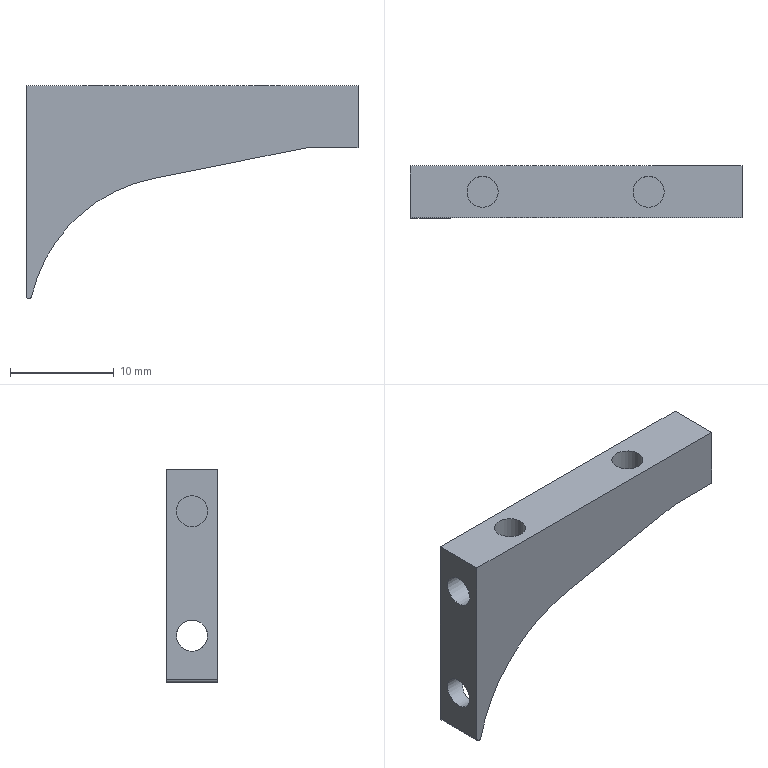Part | STEP file | 1-28.5 | 1 solid | 18 faces | box 32 x 5 x 20.5 mm | volume 1373 mm3 | plane 11 | cylinder 7 | commonest cylinder face diameters 3 x4 0.5 x2 30 x1
STEP:
#1=CARTESIAN_POINT('',(0.,0.,0.));
#2=DIRECTION('',(0.,0.,1.));
#3=DIRECTION('',(1.,0.,0.));
#4=AXIS2_PLACEMENT_3D('',#1,#2,#3);
#5=CARTESIAN_POINT('',(12.205,-2.5,11.528));
#6=VERTEX_POINT('',#5);
#7=CARTESIAN_POINT('',(27.,-2.5,14.5));
#8=VERTEX_POINT('',#7);
#9=CARTESIAN_POINT('',(12.205,-2.5,11.528));
#10=DIRECTION('',(0.9804,0.,0.1969));
#11=VECTOR('',#10,1.);
#12=LINE('',#9,#11);
#13=CARTESIAN_POINT('',(19.603,0.,13.014));
#14=DIRECTION('',(-0.1969,0.,0.9804));
#15=DIRECTION('',(0.9804,0.,0.1969));
#16=AXIS2_PLACEMENT_3D('',#13,#14,#15);
#17=PLANE('',#16);
#18=CARTESIAN_POINT('',(-7.545,-2.5));
#19=DIRECTION('',(1.,0.));
#20=VECTOR('',#19,1.);
#21=LINE('',#18,#20);
#22=(GEOMETRIC_REPRESENTATION_CONTEXT(2)PARAMETRIC_REPRESENTATION_CONTEXT()REPRESENTATION_CONTEXT('',''));
#23=DEFINITIONAL_REPRESENTATION('',(#21),#22);
#24=PCURVE('',#17,#23);
#25=CARTESIAN_POINT('',(16.,-2.5,16.));
#26=DIRECTION('',(0.,-1.,0.));
#27=DIRECTION('',(1.,0.,0.));
#28=AXIS2_PLACEMENT_3D('',#25,#26,#27);
#29=PLANE('',#28);
#30=CARTESIAN_POINT('',(-3.795,-4.472));
#31=DIRECTION('',(0.9804,0.1969));
#32=VECTOR('',#31,1.);
#33=LINE('',#30,#32);
#34=(GEOMETRIC_REPRESENTATION_CONTEXT(2)PARAMETRIC_REPRESENTATION_CONTEXT()REPRESENTATION_CONTEXT('',''));
#35=DEFINITIONAL_REPRESENTATION('',(#33),#34);
#36=PCURVE('',#29,#35);
#37=SURFACE_CURVE('',#12,(#24,#36),.PCURVE_S1.);
#38=EDGE_CURVE('',#6,#8,#37,.T.);
#39=ORIENTED_EDGE('',*,*,#38,.T.);
#40=CARTESIAN_POINT('',(27.,2.5,14.5));
#41=VERTEX_POINT('',#40);
#42=CARTESIAN_POINT('',(27.,-2.5,14.5));
#43=DIRECTION('',(0.,1.,0.));
#44=VECTOR('',#43,1.);
#45=LINE('',#42,#44);
#46=CARTESIAN_POINT('',(7.545,-2.5));
#47=DIRECTION('',(0.,1.));
#48=VECTOR('',#47,1.);
#49=LINE('',#46,#48);
#50=(GEOMETRIC_REPRESENTATION_CONTEXT(2)PARAMETRIC_REPRESENTATION_CONTEXT()REPRESENTATION_CONTEXT('',''));
#51=DEFINITIONAL_REPRESENTATION('',(#49),#50);
#52=PCURVE('',#17,#51);
#53=CARTESIAN_POINT('',(29.5,0.,14.5));
#54=DIRECTION('',(0.,0.,1.));
#55=DIRECTION('',(1.,0.,0.));
#56=AXIS2_PLACEMENT_3D('',#53,#54,#55);
#57=PLANE('',#56);
#58=CARTESIAN_POINT('',(-2.5,-2.5));
#59=DIRECTION('',(0.,1.));
#60=VECTOR('',#59,1.);
#61=LINE('',#58,#60);
#62=(GEOMETRIC_REPRESENTATION_CONTEXT(2)PARAMETRIC_REPRESENTATION_CONTEXT()REPRESENTATION_CONTEXT('',''));
#63=DEFINITIONAL_REPRESENTATION('',(#61),#62);
#64=PCURVE('',#57,#63);
#65=SURFACE_CURVE('',#45,(#52,#64),.PCURVE_S1.);
#66=EDGE_CURVE('',#8,#41,#65,.T.);
#67=ORIENTED_EDGE('',*,*,#66,.T.);
#68=CARTESIAN_POINT('',(12.205,2.5,11.528));
#69=VERTEX_POINT('',#68);
#70=CARTESIAN_POINT('',(12.205,2.5,11.528));
#71=DIRECTION('',(0.9804,0.,0.1969));
#72=VECTOR('',#71,1.);
#73=LINE('',#70,#72);
#74=CARTESIAN_POINT('',(-7.545,2.5));
#75=DIRECTION('',(1.,0.));
#76=VECTOR('',#75,1.);
#77=LINE('',#74,#76);
#78=(GEOMETRIC_REPRESENTATION_CONTEXT(2)PARAMETRIC_REPRESENTATION_CONTEXT()REPRESENTATION_CONTEXT('',''));
#79=DEFINITIONAL_REPRESENTATION('',(#77),#78);
#80=PCURVE('',#17,#79);
#81=CARTESIAN_POINT('',(16.,2.5,16.));
#82=DIRECTION('',(0.,-1.,0.));
#83=DIRECTION('',(1.,0.,0.));
#84=AXIS2_PLACEMENT_3D('',#81,#82,#83);
#85=PLANE('',#84);
#86=CARTESIAN_POINT('',(-3.795,-4.472));
#87=DIRECTION('',(0.9804,0.1969));
#88=VECTOR('',#87,1.);
#89=LINE('',#86,#88);
#90=(GEOMETRIC_REPRESENTATION_CONTEXT(2)PARAMETRIC_REPRESENTATION_CONTEXT()REPRESENTATION_CONTEXT('',''));
#91=DEFINITIONAL_REPRESENTATION('',(#89),#90);
#92=PCURVE('',#85,#91);
#93=SURFACE_CURVE('',#73,(#80,#92),.PCURVE_S1.);
#94=EDGE_CURVE('',#69,#41,#93,.T.);
#95=ORIENTED_EDGE('',*,*,#94,.F.);
#96=CARTESIAN_POINT('',(12.205,-2.5,11.528));
#97=DIRECTION('',(0.,1.,0.));
#98=VECTOR('',#97,1.);
#99=LINE('',#96,#98);
#100=CARTESIAN_POINT('',(-7.545,-2.5));
#101=DIRECTION('',(0.,1.));
#102=VECTOR('',#101,1.);
#103=LINE('',#100,#102);
#104=(GEOMETRIC_REPRESENTATION_CONTEXT(2)PARAMETRIC_REPRESENTATION_CONTEXT()REPRESENTATION_CONTEXT('',''));
#105=DEFINITIONAL_REPRESENTATION('',(#103),#104);
#106=PCURVE('',#17,#105);
#107=CARTESIAN_POINT('',(15.159,-2.5,-3.178));
#108=DIRECTION('',(0.,1.,0.));
#109=DIRECTION('',(-0.9773,0.,0.2119));
#110=AXIS2_PLACEMENT_3D('',#107,#108,#109);
#111=CYLINDRICAL_SURFACE('',#110,15.);
#112=CARTESIAN_POINT('',(1.159,0.));
#113=DIRECTION('',(0.,1.));
#114=VECTOR('',#113,1.);
#115=LINE('',#112,#114);
#116=(GEOMETRIC_REPRESENTATION_CONTEXT(2)PARAMETRIC_REPRESENTATION_CONTEXT()REPRESENTATION_CONTEXT('',''));
#117=DEFINITIONAL_REPRESENTATION('',(#115),#116);
#118=PCURVE('',#111,#117);
#119=SURFACE_CURVE('',#99,(#106,#118),.PCURVE_S1.);
#120=EDGE_CURVE('',#6,#69,#119,.T.);
#121=ORIENTED_EDGE('',*,*,#120,.F.);
#122=EDGE_LOOP('',(#39,#67,#95,#121));
#123=FACE_BOUND('',#122,.F.);
#124=ADVANCED_FACE('',(#123),#17,.F.);
#125=CARTESIAN_POINT('',(32.,-2.5,14.5));
#126=VERTEX_POINT('',#125);
#127=CARTESIAN_POINT('',(27.,-2.5,14.5));
#128=DIRECTION('',(1.,0.,0.));
#129=VECTOR('',#128,1.);
#130=LINE('',#127,#129);
#131=CARTESIAN_POINT('',(-2.5,-2.5));
#132=DIRECTION('',(1.,0.));
#133=VECTOR('',#132,1.);
#134=LINE('',#131,#133);
#135=(GEOMETRIC_REPRESENTATION_CONTEXT(2)PARAMETRIC_REPRESENTATION_CONTEXT()REPRESENTATION_CONTEXT('',''));
#136=DEFINITIONAL_REPRESENTATION('',(#134),#135);
#137=PCURVE('',#57,#136);
#138=CARTESIAN_POINT('',(11.,-1.5));
#139=DIRECTION('',(1.,0.));
#140=VECTOR('',#139,1.);
#141=LINE('',#138,#140);
#142=(GEOMETRIC_REPRESENTATION_CONTEXT(2)PARAMETRIC_REPRESENTATION_CONTEXT()REPRESENTATION_CONTEXT('',''));
#143=DEFINITIONAL_REPRESENTATION('',(#141),#142);
#144=PCURVE('',#29,#143);
#145=SURFACE_CURVE('',#130,(#137,#144),.PCURVE_S1.);
#146=EDGE_CURVE('',#8,#126,#145,.T.);
#147=ORIENTED_EDGE('',*,*,#146,.T.);
#148=CARTESIAN_POINT('',(32.,2.5,14.5));
#149=VERTEX_POINT('',#148);
#150=CARTESIAN_POINT('',(32.,-2.5,14.5));
#151=DIRECTION('',(0.,1.,0.));
#152=VECTOR('',#151,1.);
#153=LINE('',#150,#152);
#154=CARTESIAN_POINT('',(2.5,-2.5));
#155=DIRECTION('',(0.,1.));
#156=VECTOR('',#155,1.);
#157=LINE('',#154,#156);
#158=(GEOMETRIC_REPRESENTATION_CONTEXT(2)PARAMETRIC_REPRESENTATION_CONTEXT()REPRESENTATION_CONTEXT('',''));
#159=DEFINITIONAL_REPRESENTATION('',(#157),#158);
#160=PCURVE('',#57,#159);
#161=CARTESIAN_POINT('',(32.,0.,17.5));
#162=DIRECTION('',(-1.,0.,0.));
#163=DIRECTION('',(0.,0.,1.));
#164=AXIS2_PLACEMENT_3D('',#161,#162,#163);
#165=PLANE('',#164);
#166=CARTESIAN_POINT('',(-3.,-2.5));
#167=DIRECTION('',(0.,1.));
#168=VECTOR('',#167,1.);
#169=LINE('',#166,#168);
#170=(GEOMETRIC_REPRESENTATION_CONTEXT(2)PARAMETRIC_REPRESENTATION_CONTEXT()REPRESENTATION_CONTEXT('',''));
#171=DEFINITIONAL_REPRESENTATION('',(#169),#170);
#172=PCURVE('',#165,#171);
#173=SURFACE_CURVE('',#153,(#160,#172),.PCURVE_S1.);
#174=EDGE_CURVE('',#126,#149,#173,.T.);
#175=ORIENTED_EDGE('',*,*,#174,.T.);
#176=CARTESIAN_POINT('',(27.,2.5,14.5));
#177=DIRECTION('',(1.,0.,0.));
#178=VECTOR('',#177,1.);
#179=LINE('',#176,#178);
#180=CARTESIAN_POINT('',(-2.5,2.5));
#181=DIRECTION('',(1.,0.));
#182=VECTOR('',#181,1.);
#183=LINE('',#180,#182);
#184=(GEOMETRIC_REPRESENTATION_CONTEXT(2)PARAMETRIC_REPRESENTATION_CONTEXT()REPRESENTATION_CONTEXT('',''));
#185=DEFINITIONAL_REPRESENTATION('',(#183),#184);
#186=PCURVE('',#57,#185);
#187=CARTESIAN_POINT('',(11.,-1.5));
#188=DIRECTION('',(1.,0.));
#189=VECTOR('',#188,1.);
#190=LINE('',#187,#189);
#191=(GEOMETRIC_REPRESENTATION_CONTEXT(2)PARAMETRIC_REPRESENTATION_CONTEXT()REPRESENTATION_CONTEXT('',''));
#192=DEFINITIONAL_REPRESENTATION('',(#190),#191);
#193=PCURVE('',#85,#192);
#194=SURFACE_CURVE('',#179,(#186,#193),.PCURVE_S1.);
#195=EDGE_CURVE('',#41,#149,#194,.T.);
#196=ORIENTED_EDGE('',*,*,#195,.F.);
#197=ORIENTED_EDGE('',*,*,#66,.F.);
#198=EDGE_LOOP('',(#147,#175,#196,#197));
#199=FACE_BOUND('',#198,.F.);
#200=ADVANCED_FACE('',(#199),#57,.F.);
#201=CARTESIAN_POINT('',(32.,-2.5,20.5));
#202=VERTEX_POINT('',#201);
#203=CARTESIAN_POINT('',(32.,-2.5,14.5));
#204=DIRECTION('',(0.,0.,1.));
#205=VECTOR('',#204,1.);
#206=LINE('',#203,#205);
#207=CARTESIAN_POINT('',(-3.,-2.5));
#208=DIRECTION('',(1.,0.));
#209=VECTOR('',#208,1.);
#210=LINE('',#207,#209);
#211=(GEOMETRIC_REPRESENTATION_CONTEXT(2)PARAMETRIC_REPRESENTATION_CONTEXT()REPRESENTATION_CONTEXT('',''));
#212=DEFINITIONAL_REPRESENTATION('',(#210),#211);
#213=PCURVE('',#165,#212);
#214=CARTESIAN_POINT('',(16.,-1.5));
#215=DIRECTION('',(0.,1.));
#216=VECTOR('',#215,1.);
#217=LINE('',#214,#216);
#218=(GEOMETRIC_REPRESENTATION_CONTEXT(2)PARAMETRIC_REPRESENTATION_CONTEXT()REPRESENTATION_CONTEXT('',''));
#219=DEFINITIONAL_REPRESENTATION('',(#217),#218);
#220=PCURVE('',#29,#219);
#221=SURFACE_CURVE('',#206,(#213,#220),.PCURVE_S1.);
#222=EDGE_CURVE('',#126,#202,#221,.T.);
#223=ORIENTED_EDGE('',*,*,#222,.T.);
#224=CARTESIAN_POINT('',(32.,2.5,20.5));
#225=VERTEX_POINT('',#224);
#226=CARTESIAN_POINT('',(32.,-2.5,20.5));
#227=DIRECTION('',(0.,1.,0.));
#228=VECTOR('',#227,1.);
#229=LINE('',#226,#228);
#230=CARTESIAN_POINT('',(3.,-2.5));
#231=DIRECTION('',(0.,1.));
#232=VECTOR('',#231,1.);
#233=LINE('',#230,#232);
#234=(GEOMETRIC_REPRESENTATION_CONTEXT(2)PARAMETRIC_REPRESENTATION_CONTEXT()REPRESENTATION_CONTEXT('',''));
#235=DEFINITIONAL_REPRESENTATION('',(#233),#234);
#236=PCURVE('',#165,#235);
#237=CARTESIAN_POINT('',(16.,0.,20.5));
#238=DIRECTION('',(0.,0.,-1.));
#239=DIRECTION('',(-1.,0.,0.));
#240=AXIS2_PLACEMENT_3D('',#237,#238,#239);
#241=PLANE('',#240);
#242=CARTESIAN_POINT('',(-16.,-2.5));
#243=DIRECTION('',(0.,1.));
#244=VECTOR('',#243,1.);
#245=LINE('',#242,#244);
#246=(GEOMETRIC_REPRESENTATION_CONTEXT(2)PARAMETRIC_REPRESENTATION_CONTEXT()REPRESENTATION_CONTEXT('',''));
#247=DEFINITIONAL_REPRESENTATION('',(#245),#246);
#248=PCURVE('',#241,#247);
#249=SURFACE_CURVE('',#229,(#236,#248),.PCURVE_S1.);
#250=EDGE_CURVE('',#202,#225,#249,.T.);
#251=ORIENTED_EDGE('',*,*,#250,.T.);
#252=CARTESIAN_POINT('',(32.,2.5,14.5));
#253=DIRECTION('',(0.,0.,1.));
#254=VECTOR('',#253,1.);
#255=LINE('',#252,#254);
#256=CARTESIAN_POINT('',(-3.,2.5));
#257=DIRECTION('',(1.,0.));
#258=VECTOR('',#257,1.);
#259=LINE('',#256,#258);
#260=(GEOMETRIC_REPRESENTATION_CONTEXT(2)PARAMETRIC_REPRESENTATION_CONTEXT()REPRESENTATION_CONTEXT('',''));
#261=DEFINITIONAL_REPRESENTATION('',(#259),#260);
#262=PCURVE('',#165,#261);
#263=CARTESIAN_POINT('',(16.,-1.5));
#264=DIRECTION('',(0.,1.));
#265=VECTOR('',#264,1.);
#266=LINE('',#263,#265);
#267=(GEOMETRIC_REPRESENTATION_CONTEXT(2)PARAMETRIC_REPRESENTATION_CONTEXT()REPRESENTATION_CONTEXT('',''));
#268=DEFINITIONAL_REPRESENTATION('',(#266),#267);
#269=PCURVE('',#85,#268);
#270=SURFACE_CURVE('',#255,(#262,#269),.PCURVE_S1.);
#271=EDGE_CURVE('',#149,#225,#270,.T.);
#272=ORIENTED_EDGE('',*,*,#271,.F.);
#273=ORIENTED_EDGE('',*,*,#174,.F.);
#274=EDGE_LOOP('',(#223,#251,#272,#273));
#275=FACE_BOUND('',#274,.F.);
#276=ADVANCED_FACE('',(#275),#165,.F.);
#277=ORIENTED_EDGE('',*,*,#38,.T.);
#278=ORIENTED_EDGE('',*,*,#146,.T.);
#279=ORIENTED_EDGE('',*,*,#222,.T.);
#280=CARTESIAN_POINT('',(0.,-2.5,20.5));
#281=VERTEX_POINT('',#280);
#282=CARTESIAN_POINT('',(32.,-2.5,20.5));
#283=DIRECTION('',(-1.,0.,0.));
#284=VECTOR('',#283,1.);
#285=LINE('',#282,#284);
#286=CARTESIAN_POINT('',(16.,4.5));
#287=DIRECTION('',(-1.,0.));
#288=VECTOR('',#287,1.);
#289=LINE('',#286,#288);
#290=(GEOMETRIC_REPRESENTATION_CONTEXT(2)PARAMETRIC_REPRESENTATION_CONTEXT()REPRESENTATION_CONTEXT('',''));
#291=DEFINITIONAL_REPRESENTATION('',(#289),#290);
#292=PCURVE('',#29,#291);
#293=CARTESIAN_POINT('',(-16.,-2.5));
#294=DIRECTION('',(1.,0.));
#295=VECTOR('',#294,1.);
#296=LINE('',#293,#295);
#297=(GEOMETRIC_REPRESENTATION_CONTEXT(2)PARAMETRIC_REPRESENTATION_CONTEXT()REPRESENTATION_CONTEXT('',''));
#298=DEFINITIONAL_REPRESENTATION('',(#296),#297);
#299=PCURVE('',#241,#298);
#300=SURFACE_CURVE('',#285,(#292,#299),.PCURVE_S1.);
#301=EDGE_CURVE('',#202,#281,#300,.T.);
#302=ORIENTED_EDGE('',*,*,#301,.T.);
#303=CARTESIAN_POINT('',(0.,-2.5,0.25));
#304=VERTEX_POINT('',#303);
#305=CARTESIAN_POINT('',(0.,-2.5,20.5));
#306=DIRECTION('',(0.,0.,-1.));
#307=VECTOR('',#306,1.);
#308=LINE('',#305,#307);
#309=CARTESIAN_POINT('',(-16.,4.5));
#310=DIRECTION('',(0.,-1.));
#311=VECTOR('',#310,1.);
#312=LINE('',#309,#311);
#313=(GEOMETRIC_REPRESENTATION_CONTEXT(2)PARAMETRIC_REPRESENTATION_CONTEXT()REPRESENTATION_CONTEXT('',''));
#314=DEFINITIONAL_REPRESENTATION('',(#312),#313);
#315=PCURVE('',#29,#314);
#316=CARTESIAN_POINT('',(0.,0.,10.25));
#317=DIRECTION('',(1.,0.,0.));
#318=DIRECTION('',(0.,0.,-1.));
#319=AXIS2_PLACEMENT_3D('',#316,#317,#318);
#320=PLANE('',#319);
#321=CARTESIAN_POINT('',(-10.25,-2.5));
#322=DIRECTION('',(1.,0.));
#323=VECTOR('',#322,1.);
#324=LINE('',#321,#323);
#325=(GEOMETRIC_REPRESENTATION_CONTEXT(2)PARAMETRIC_REPRESENTATION_CONTEXT()REPRESENTATION_CONTEXT('',''));
#326=DEFINITIONAL_REPRESENTATION('',(#324),#325);
#327=PCURVE('',#320,#326);
#328=SURFACE_CURVE('',#308,(#315,#327),.PCURVE_S1.);
#329=EDGE_CURVE('',#281,#304,#328,.T.);
#330=ORIENTED_EDGE('',*,*,#329,.T.);
#331=CARTESIAN_POINT('',(0.25,-2.5,0.));
#332=VERTEX_POINT('',#331);
#333=CARTESIAN_POINT('',(0.25,-2.5,0.25));
#334=DIRECTION('',(0.,-1.,0.));
#335=DIRECTION('',(-1.,0.,0.));
#336=AXIS2_PLACEMENT_3D('',#333,#334,#335);
#337=CIRCLE('',#336,0.25);
#338=CARTESIAN_POINT('',(-15.75,-15.75));
#339=DIRECTION('',(-1.,0.));
#340=AXIS2_PLACEMENT_2D('',#338,#339);
#341=CIRCLE('',#340,0.25);
#342=(GEOMETRIC_REPRESENTATION_CONTEXT(2)PARAMETRIC_REPRESENTATION_CONTEXT()REPRESENTATION_CONTEXT('',''));
#343=DEFINITIONAL_REPRESENTATION('',(#341),#342);
#344=PCURVE('',#29,#343);
#345=CARTESIAN_POINT('',(0.25,-2.5,0.25));
#346=DIRECTION('',(0.,1.,0.));
#347=DIRECTION('',(-1.,0.,0.));
#348=AXIS2_PLACEMENT_3D('',#345,#346,#347);
#349=CYLINDRICAL_SURFACE('',#348,0.25);
#350=CARTESIAN_POINT('',(6.283,0.));
#351=DIRECTION('',(-1.,0.));
#352=VECTOR('',#351,1.);
#353=LINE('',#350,#352);
#354=(GEOMETRIC_REPRESENTATION_CONTEXT(2)PARAMETRIC_REPRESENTATION_CONTEXT()REPRESENTATION_CONTEXT('',''));
#355=DEFINITIONAL_REPRESENTATION('',(#353),#354);
#356=PCURVE('',#349,#355);
#357=SURFACE_CURVE('',#337,(#344,#356),.PCURVE_S1.);
#358=EDGE_CURVE('',#304,#332,#357,.T.);
#359=ORIENTED_EDGE('',*,*,#358,.T.);
#360=CARTESIAN_POINT('',(0.2998,-2.5,0.));
#361=VERTEX_POINT('',#360);
#362=CARTESIAN_POINT('',(0.25,-2.5,0.));
#363=DIRECTION('',(1.,0.,0.));
#364=VECTOR('',#363,1.);
#365=LINE('',#362,#364);
#366=CARTESIAN_POINT('',(-15.75,-16.));
#367=DIRECTION('',(1.,0.));
#368=VECTOR('',#367,1.);
#369=LINE('',#366,#368);
#370=(GEOMETRIC_REPRESENTATION_CONTEXT(2)PARAMETRIC_REPRESENTATION_CONTEXT()REPRESENTATION_CONTEXT('',''));
#371=DEFINITIONAL_REPRESENTATION('',(#369),#370);
#372=PCURVE('',#29,#371);
#373=CARTESIAN_POINT('',(0.25,0.,0.));
#374=DIRECTION('',(0.,0.,1.));
#375=DIRECTION('',(1.,0.,0.));
#376=AXIS2_PLACEMENT_3D('',#373,#374,#375);
#377=PLANE('',#376);
#378=CARTESIAN_POINT('',(0.,-2.5));
#379=DIRECTION('',(1.,0.));
#380=VECTOR('',#379,1.);
#381=LINE('',#378,#380);
#382=(GEOMETRIC_REPRESENTATION_CONTEXT(2)PARAMETRIC_REPRESENTATION_CONTEXT()REPRESENTATION_CONTEXT('',''));
#383=DEFINITIONAL_REPRESENTATION('',(#381),#382);
#384=PCURVE('',#377,#383);
#385=SURFACE_CURVE('',#365,(#372,#384),.PCURVE_S1.);
#386=EDGE_CURVE('',#332,#361,#385,.T.);
#387=ORIENTED_EDGE('',*,*,#386,.T.);
#388=CARTESIAN_POINT('',(0.5434,-2.5,0.1938));
#389=VERTEX_POINT('',#388);
#390=CARTESIAN_POINT('',(0.2998,-2.5,0.25));
#391=DIRECTION('',(0.,-1.,0.));
#392=DIRECTION('',(0.,0.,-1.));
#393=AXIS2_PLACEMENT_3D('',#390,#391,#392);
#394=CIRCLE('',#393,0.25);
#395=CARTESIAN_POINT('',(-15.7,-15.75));
#396=DIRECTION('',(0.,-1.));
#397=AXIS2_PLACEMENT_2D('',#395,#396);
#398=CIRCLE('',#397,0.25);
#399=(GEOMETRIC_REPRESENTATION_CONTEXT(2)PARAMETRIC_REPRESENTATION_CONTEXT()REPRESENTATION_CONTEXT('',''));
#400=DEFINITIONAL_REPRESENTATION('',(#398),#399);
#401=PCURVE('',#29,#400);
#402=CARTESIAN_POINT('',(0.2998,-2.5,0.25));
#403=DIRECTION('',(0.,1.,0.));
#404=DIRECTION('',(0.,0.,-1.));
#405=AXIS2_PLACEMENT_3D('',#402,#403,#404);
#406=CYLINDRICAL_SURFACE('',#405,0.25);
#407=CARTESIAN_POINT('',(6.283,0.));
#408=DIRECTION('',(-1.,0.));
#409=VECTOR('',#408,1.);
#410=LINE('',#407,#409);
#411=(GEOMETRIC_REPRESENTATION_CONTEXT(2)PARAMETRIC_REPRESENTATION_CONTEXT()REPRESENTATION_CONTEXT('',''));
#412=DEFINITIONAL_REPRESENTATION('',(#410),#411);
#413=PCURVE('',#406,#412);
#414=SURFACE_CURVE('',#394,(#401,#413),.PCURVE_S1.);
#415=EDGE_CURVE('',#361,#389,#414,.T.);
#416=ORIENTED_EDGE('',*,*,#415,.T.);
#417=CARTESIAN_POINT('',(15.159,-2.5,-3.178));
#418=DIRECTION('',(0.,1.,0.));
#419=DIRECTION('',(-0.9744,0.,0.2248));
#420=AXIS2_PLACEMENT_3D('',#417,#418,#419);
#421=CIRCLE('',#420,15.);
#422=CARTESIAN_POINT('',(-15.457,-15.806));
#423=CARTESIAN_POINT('',(-9.616,9.51));
#424=CARTESIAN_POINT('',(9.388,-8.206));
#425=CARTESIAN_POINT('',(28.392,-25.922));
#426=CARTESIAN_POINT('',(3.547,-33.522));
#427=CARTESIAN_POINT('',(-21.297,-41.122));
#428=CARTESIAN_POINT('',(-15.457,-15.806));
#429=(BOUNDED_CURVE()B_SPLINE_CURVE(2,(#422,#423,#424,#425,#426,#427,#428),.UNSPECIFIED.,.T.,.F.)B_SPLINE_CURVE_WITH_KNOTS((1,2,2,2,2,1),(-2.094,0.,2.094,4.189,6.283,8.378),.UNSPECIFIED.)CURVE()GEOMETRIC_REPRESENTATION_ITEM()RATIONAL_B_SPLINE_CURVE((1.,0.5,1.,0.5,1.,0.5,1.))REPRESENTATION_ITEM(''));
#430=(GEOMETRIC_REPRESENTATION_CONTEXT(2)PARAMETRIC_REPRESENTATION_CONTEXT()REPRESENTATION_CONTEXT('',''));
#431=DEFINITIONAL_REPRESENTATION('',(#429),#430);
#432=PCURVE('',#29,#431);
#433=CARTESIAN_POINT('',(0.01324,0.));
#434=DIRECTION('',(1.,0.));
#435=VECTOR('',#434,1.);
#436=LINE('',#433,#435);
#437=(GEOMETRIC_REPRESENTATION_CONTEXT(2)PARAMETRIC_REPRESENTATION_CONTEXT()REPRESENTATION_CONTEXT('',''));
#438=DEFINITIONAL_REPRESENTATION('',(#436),#437);
#439=PCURVE('',#111,#438);
#440=SURFACE_CURVE('',#421,(#432,#439),.PCURVE_S1.);
#441=EDGE_CURVE('',#389,#6,#440,.T.);
#442=ORIENTED_EDGE('',*,*,#441,.T.);
#443=EDGE_LOOP('',(#277,#278,#279,#302,#330,#359,#387,#416,#442));
#444=FACE_BOUND('',#443,.T.);
#445=ADVANCED_FACE('',(#444),#29,.T.);
#446=ORIENTED_EDGE('',*,*,#94,.T.);
#447=ORIENTED_EDGE('',*,*,#195,.T.);
#448=ORIENTED_EDGE('',*,*,#271,.T.);
#449=CARTESIAN_POINT('',(0.,2.5,20.5));
#450=VERTEX_POINT('',#449);
#451=CARTESIAN_POINT('',(32.,2.5,20.5));
#452=DIRECTION('',(-1.,0.,0.));
#453=VECTOR('',#452,1.);
#454=LINE('',#451,#453);
#455=CARTESIAN_POINT('',(16.,4.5));
#456=DIRECTION('',(-1.,0.));
#457=VECTOR('',#456,1.);
#458=LINE('',#455,#457);
#459=(GEOMETRIC_REPRESENTATION_CONTEXT(2)PARAMETRIC_REPRESENTATION_CONTEXT()REPRESENTATION_CONTEXT('',''));
#460=DEFINITIONAL_REPRESENTATION('',(#458),#459);
#461=PCURVE('',#85,#460);
#462=CARTESIAN_POINT('',(-16.,2.5));
#463=DIRECTION('',(1.,0.));
#464=VECTOR('',#463,1.);
#465=LINE('',#462,#464);
#466=(GEOMETRIC_REPRESENTATION_CONTEXT(2)PARAMETRIC_REPRESENTATION_CONTEXT()REPRESENTATION_CONTEXT('',''));
#467=DEFINITIONAL_REPRESENTATION('',(#465),#466);
#468=PCURVE('',#241,#467);
#469=SURFACE_CURVE('',#454,(#461,#468),.PCURVE_S1.);
#470=EDGE_CURVE('',#225,#450,#469,.T.);
#471=ORIENTED_EDGE('',*,*,#470,.T.);
#472=CARTESIAN_POINT('',(0.,2.5,0.25));
#473=VERTEX_POINT('',#472);
#474=CARTESIAN_POINT('',(0.,2.5,20.5));
#475=DIRECTION('',(0.,0.,-1.));
#476=VECTOR('',#475,1.);
#477=LINE('',#474,#476);
#478=CARTESIAN_POINT('',(-16.,4.5));
#479=DIRECTION('',(0.,-1.));
#480=VECTOR('',#479,1.);
#481=LINE('',#478,#480);
#482=(GEOMETRIC_REPRESENTATION_CONTEXT(2)PARAMETRIC_REPRESENTATION_CONTEXT()REPRESENTATION_CONTEXT('',''));
#483=DEFINITIONAL_REPRESENTATION('',(#481),#482);
#484=PCURVE('',#85,#483);
#485=CARTESIAN_POINT('',(-10.25,2.5));
#486=DIRECTION('',(1.,0.));
#487=VECTOR('',#486,1.);
#488=LINE('',#485,#487);
#489=(GEOMETRIC_REPRESENTATION_CONTEXT(2)PARAMETRIC_REPRESENTATION_CONTEXT()REPRESENTATION_CONTEXT('',''));
#490=DEFINITIONAL_REPRESENTATION('',(#488),#489);
#491=PCURVE('',#320,#490);
#492=SURFACE_CURVE('',#477,(#484,#491),.PCURVE_S1.);
#493=EDGE_CURVE('',#450,#473,#492,.T.);
#494=ORIENTED_EDGE('',*,*,#493,.T.);
#495=CARTESIAN_POINT('',(0.25,2.5,0.));
#496=VERTEX_POINT('',#495);
#497=CARTESIAN_POINT('',(0.25,2.5,0.25));
#498=DIRECTION('',(0.,-1.,0.));
#499=DIRECTION('',(-1.,0.,0.));
#500=AXIS2_PLACEMENT_3D('',#497,#498,#499);
#501=CIRCLE('',#500,0.25);
#502=CARTESIAN_POINT('',(-15.75,-15.75));
#503=DIRECTION('',(-1.,0.));
#504=AXIS2_PLACEMENT_2D('',#502,#503);
#505=CIRCLE('',#504,0.25);
#506=(GEOMETRIC_REPRESENTATION_CONTEXT(2)PARAMETRIC_REPRESENTATION_CONTEXT()REPRESENTATION_CONTEXT('',''));
#507=DEFINITIONAL_REPRESENTATION('',(#505),#506);
#508=PCURVE('',#85,#507);
#509=CARTESIAN_POINT('',(6.283,5.));
#510=DIRECTION('',(-1.,0.));
#511=VECTOR('',#510,1.);
#512=LINE('',#509,#511);
#513=(GEOMETRIC_REPRESENTATION_CONTEXT(2)PARAMETRIC_REPRESENTATION_CONTEXT()REPRESENTATION_CONTEXT('',''));
#514=DEFINITIONAL_REPRESENTATION('',(#512),#513);
#515=PCURVE('',#349,#514);
#516=SURFACE_CURVE('',#501,(#508,#515),.PCURVE_S1.);
#517=EDGE_CURVE('',#473,#496,#516,.T.);
#518=ORIENTED_EDGE('',*,*,#517,.T.);
#519=CARTESIAN_POINT('',(0.2998,2.5,0.));
#520=VERTEX_POINT('',#519);
#521=CARTESIAN_POINT('',(0.25,2.5,0.));
#522=DIRECTION('',(1.,0.,0.));
#523=VECTOR('',#522,1.);
#524=LINE('',#521,#523);
#525=CARTESIAN_POINT('',(-15.75,-16.));
#526=DIRECTION('',(1.,0.));
#527=VECTOR('',#526,1.);
#528=LINE('',#525,#527);
#529=(GEOMETRIC_REPRESENTATION_CONTEXT(2)PARAMETRIC_REPRESENTATION_CONTEXT()REPRESENTATION_CONTEXT('',''));
#530=DEFINITIONAL_REPRESENTATION('',(#528),#529);
#531=PCURVE('',#85,#530);
#532=CARTESIAN_POINT('',(0.,2.5));
#533=DIRECTION('',(1.,0.));
#534=VECTOR('',#533,1.);
#535=LINE('',#532,#534);
#536=(GEOMETRIC_REPRESENTATION_CONTEXT(2)PARAMETRIC_REPRESENTATION_CONTEXT()REPRESENTATION_CONTEXT('',''));
#537=DEFINITIONAL_REPRESENTATION('',(#535),#536);
#538=PCURVE('',#377,#537);
#539=SURFACE_CURVE('',#524,(#531,#538),.PCURVE_S1.);
#540=EDGE_CURVE('',#496,#520,#539,.T.);
#541=ORIENTED_EDGE('',*,*,#540,.T.);
#542=CARTESIAN_POINT('',(0.5434,2.5,0.1938));
#543=VERTEX_POINT('',#542);
#544=CARTESIAN_POINT('',(0.2998,2.5,0.25));
#545=DIRECTION('',(0.,-1.,0.));
#546=DIRECTION('',(0.,0.,-1.));
#547=AXIS2_PLACEMENT_3D('',#544,#545,#546);
#548=CIRCLE('',#547,0.25);
#549=CARTESIAN_POINT('',(-15.7,-15.75));
#550=DIRECTION('',(0.,-1.));
#551=AXIS2_PLACEMENT_2D('',#549,#550);
#552=CIRCLE('',#551,0.25);
#553=(GEOMETRIC_REPRESENTATION_CONTEXT(2)PARAMETRIC_REPRESENTATION_CONTEXT()REPRESENTATION_CONTEXT('',''));
#554=DEFINITIONAL_REPRESENTATION('',(#552),#553);
#555=PCURVE('',#85,#554);
#556=CARTESIAN_POINT('',(6.283,5.));
#557=DIRECTION('',(-1.,0.));
#558=VECTOR('',#557,1.);
#559=LINE('',#556,#558);
#560=(GEOMETRIC_REPRESENTATION_CONTEXT(2)PARAMETRIC_REPRESENTATION_CONTEXT()REPRESENTATION_CONTEXT('',''));
#561=DEFINITIONAL_REPRESENTATION('',(#559),#560);
#562=PCURVE('',#406,#561);
#563=SURFACE_CURVE('',#548,(#555,#562),.PCURVE_S1.);
#564=EDGE_CURVE('',#520,#543,#563,.T.);
#565=ORIENTED_EDGE('',*,*,#564,.T.);
#566=CARTESIAN_POINT('',(15.159,2.5,-3.178));
#567=DIRECTION('',(0.,1.,0.));
#568=DIRECTION('',(-0.9744,0.,0.2248));
#569=AXIS2_PLACEMENT_3D('',#566,#567,#568);
#570=CIRCLE('',#569,15.);
#571=CARTESIAN_POINT('',(-15.457,-15.806));
#572=CARTESIAN_POINT('',(-9.616,9.51));
#573=CARTESIAN_POINT('',(9.388,-8.206));
#574=CARTESIAN_POINT('',(28.392,-25.922));
#575=CARTESIAN_POINT('',(3.547,-33.522));
#576=CARTESIAN_POINT('',(-21.297,-41.122));
#577=CARTESIAN_POINT('',(-15.457,-15.806));
#578=(BOUNDED_CURVE()B_SPLINE_CURVE(2,(#571,#572,#573,#574,#575,#576,#577),.UNSPECIFIED.,.T.,.F.)B_SPLINE_CURVE_WITH_KNOTS((1,2,2,2,2,1),(-2.094,0.,2.094,4.189,6.283,8.378),.UNSPECIFIED.)CURVE()GEOMETRIC_REPRESENTATION_ITEM()RATIONAL_B_SPLINE_CURVE((1.,0.5,1.,0.5,1.,0.5,1.))REPRESENTATION_ITEM(''));
#579=(GEOMETRIC_REPRESENTATION_CONTEXT(2)PARAMETRIC_REPRESENTATION_CONTEXT()REPRESENTATION_CONTEXT('',''));
#580=DEFINITIONAL_REPRESENTATION('',(#578),#579);
#581=PCURVE('',#85,#580);
#582=CARTESIAN_POINT('',(0.01324,5.));
#583=DIRECTION('',(1.,0.));
#584=VECTOR('',#583,1.);
#585=LINE('',#582,#584);
#586=(GEOMETRIC_REPRESENTATION_CONTEXT(2)PARAMETRIC_REPRESENTATION_CONTEXT()REPRESENTATION_CONTEXT('',''));
#587=DEFINITIONAL_REPRESENTATION('',(#585),#586);
#588=PCURVE('',#111,#587);
#589=SURFACE_CURVE('',#570,(#581,#588),.PCURVE_S1.);
#590=EDGE_CURVE('',#543,#69,#589,.T.);
#591=ORIENTED_EDGE('',*,*,#590,.T.);
#592=EDGE_LOOP('',(#446,#447,#448,#471,#494,#518,#541,#565,#591));
#593=FACE_BOUND('',#592,.F.);
#594=ADVANCED_FACE('',(#593),#85,.F.);
#595=ORIENTED_EDGE('',*,*,#540,.F.);
#596=CARTESIAN_POINT('',(0.25,-2.5,0.));
#597=DIRECTION('',(0.,1.,0.));
#598=VECTOR('',#597,1.);
#599=LINE('',#596,#598);
#600=CARTESIAN_POINT('',(0.,-2.5));
#601=DIRECTION('',(0.,1.));
#602=VECTOR('',#601,1.);
#603=LINE('',#600,#602);
#604=(GEOMETRIC_REPRESENTATION_CONTEXT(2)PARAMETRIC_REPRESENTATION_CONTEXT()REPRESENTATION_CONTEXT('',''));
#605=DEFINITIONAL_REPRESENTATION('',(#603),#604);
#606=PCURVE('',#377,#605);
#607=CARTESIAN_POINT('',(4.712,0.));
#608=DIRECTION('',(0.,1.));
#609=VECTOR('',#608,1.);
#610=LINE('',#607,#609);
#611=(GEOMETRIC_REPRESENTATION_CONTEXT(2)PARAMETRIC_REPRESENTATION_CONTEXT()REPRESENTATION_CONTEXT('',''));
#612=DEFINITIONAL_REPRESENTATION('',(#610),#611);
#613=PCURVE('',#349,#612);
#614=SURFACE_CURVE('',#599,(#606,#613),.PCURVE_S1.);
#615=EDGE_CURVE('',#332,#496,#614,.T.);
#616=ORIENTED_EDGE('',*,*,#615,.F.);
#617=ORIENTED_EDGE('',*,*,#386,.T.);
#618=CARTESIAN_POINT('',(0.2998,-2.5,0.));
#619=DIRECTION('',(0.,1.,0.));
#620=VECTOR('',#619,1.);
#621=LINE('',#618,#620);
#622=CARTESIAN_POINT('',(0.04976,-2.5));
#623=DIRECTION('',(0.,1.));
#624=VECTOR('',#623,1.);
#625=LINE('',#622,#624);
#626=(GEOMETRIC_REPRESENTATION_CONTEXT(2)PARAMETRIC_REPRESENTATION_CONTEXT()REPRESENTATION_CONTEXT('',''));
#627=DEFINITIONAL_REPRESENTATION('',(#625),#626);
#628=PCURVE('',#377,#627);
#629=CARTESIAN_POINT('',(6.283,0.));
#630=DIRECTION('',(0.,1.));
#631=VECTOR('',#630,1.);
#632=LINE('',#629,#631);
#633=(GEOMETRIC_REPRESENTATION_CONTEXT(2)PARAMETRIC_REPRESENTATION_CONTEXT()REPRESENTATION_CONTEXT('',''));
#634=DEFINITIONAL_REPRESENTATION('',(#632),#633);
#635=PCURVE('',#406,#634);
#636=SURFACE_CURVE('',#621,(#628,#635),.PCURVE_S1.);
#637=EDGE_CURVE('',#361,#520,#636,.T.);
#638=ORIENTED_EDGE('',*,*,#637,.T.);
#639=EDGE_LOOP('',(#595,#616,#617,#638));
#640=FACE_BOUND('',#639,.F.);
#641=ADVANCED_FACE('',(#640),#377,.F.);
#642=CARTESIAN_POINT('',(0.,-2.5,0.25));
#643=DIRECTION('',(0.,1.,0.));
#644=VECTOR('',#643,1.);
#645=LINE('',#642,#644);
#646=CARTESIAN_POINT('',(6.283,0.));
#647=DIRECTION('',(0.,1.));
#648=VECTOR('',#647,1.);
#649=LINE('',#646,#648);
#650=(GEOMETRIC_REPRESENTATION_CONTEXT(2)PARAMETRIC_REPRESENTATION_CONTEXT()REPRESENTATION_CONTEXT('',''));
#651=DEFINITIONAL_REPRESENTATION('',(#649),#650);
#652=PCURVE('',#349,#651);
#653=CARTESIAN_POINT('',(10.,-2.5));
#654=DIRECTION('',(0.,1.));
#655=VECTOR('',#654,1.);
#656=LINE('',#653,#655);
#657=(GEOMETRIC_REPRESENTATION_CONTEXT(2)PARAMETRIC_REPRESENTATION_CONTEXT()REPRESENTATION_CONTEXT('',''));
#658=DEFINITIONAL_REPRESENTATION('',(#656),#657);
#659=PCURVE('',#320,#658);
#660=SURFACE_CURVE('',#645,(#652,#659),.PCURVE_S1.);
#661=EDGE_CURVE('',#304,#473,#660,.T.);
#662=ORIENTED_EDGE('',*,*,#661,.T.);
#663=ORIENTED_EDGE('',*,*,#517,.T.);
#664=ORIENTED_EDGE('',*,*,#615,.F.);
#665=ORIENTED_EDGE('',*,*,#358,.F.);
#666=EDGE_LOOP('',(#662,#663,#664,#665));
#667=FACE_BOUND('',#666,.T.);
#668=ADVANCED_FACE('',(#667),#349,.T.);
#669=ORIENTED_EDGE('',*,*,#637,.T.);
#670=ORIENTED_EDGE('',*,*,#564,.T.);
#671=CARTESIAN_POINT('',(0.5434,-2.5,0.1938));
#672=DIRECTION('',(0.,1.,0.));
#673=VECTOR('',#672,1.);
#674=LINE('',#671,#673);
#675=CARTESIAN_POINT('',(4.939,0.));
#676=DIRECTION('',(0.,1.));
#677=VECTOR('',#676,1.);
#678=LINE('',#675,#677);
#679=(GEOMETRIC_REPRESENTATION_CONTEXT(2)PARAMETRIC_REPRESENTATION_CONTEXT()REPRESENTATION_CONTEXT('',''));
#680=DEFINITIONAL_REPRESENTATION('',(#678),#679);
#681=PCURVE('',#406,#680);
#682=CARTESIAN_POINT('',(0.01324,0.));
#683=DIRECTION('',(0.,1.));
#684=VECTOR('',#683,1.);
#685=LINE('',#682,#684);
#686=(GEOMETRIC_REPRESENTATION_CONTEXT(2)PARAMETRIC_REPRESENTATION_CONTEXT()REPRESENTATION_CONTEXT('',''));
#687=DEFINITIONAL_REPRESENTATION('',(#685),#686);
#688=PCURVE('',#111,#687);
#689=SURFACE_CURVE('',#674,(#681,#688),.PCURVE_S1.);
#690=EDGE_CURVE('',#389,#543,#689,.T.);
#691=ORIENTED_EDGE('',*,*,#690,.F.);
#692=ORIENTED_EDGE('',*,*,#415,.F.);
#693=EDGE_LOOP('',(#669,#670,#691,#692));
#694=FACE_BOUND('',#693,.T.);
#695=ADVANCED_FACE('',(#694),#406,.T.);
#696=ORIENTED_EDGE('',*,*,#301,.T.);
#697=CARTESIAN_POINT('',(0.,-2.5,20.5));
#698=DIRECTION('',(0.,1.,0.));
#699=VECTOR('',#698,1.);
#700=LINE('',#697,#699);
#701=CARTESIAN_POINT('',(16.,-2.5));
#702=DIRECTION('',(0.,1.));
#703=VECTOR('',#702,1.);
#704=LINE('',#701,#703);
#705=(GEOMETRIC_REPRESENTATION_CONTEXT(2)PARAMETRIC_REPRESENTATION_CONTEXT()REPRESENTATION_CONTEXT('',''));
#706=DEFINITIONAL_REPRESENTATION('',(#704),#705);
#707=PCURVE('',#241,#706);
#708=CARTESIAN_POINT('',(-10.25,-2.5));
#709=DIRECTION('',(0.,1.));
#710=VECTOR('',#709,1.);
#711=LINE('',#708,#710);
#712=(GEOMETRIC_REPRESENTATION_CONTEXT(2)PARAMETRIC_REPRESENTATION_CONTEXT()REPRESENTATION_CONTEXT('',''));
#713=DEFINITIONAL_REPRESENTATION('',(#711),#712);
#714=PCURVE('',#320,#713);
#715=SURFACE_CURVE('',#700,(#707,#714),.PCURVE_S1.);
#716=EDGE_CURVE('',#281,#450,#715,.T.);
#717=ORIENTED_EDGE('',*,*,#716,.T.);
#718=ORIENTED_EDGE('',*,*,#470,.F.);
#719=ORIENTED_EDGE('',*,*,#250,.F.);
#720=EDGE_LOOP('',(#696,#717,#718,#719));
#721=FACE_BOUND('',#720,.F.);
#722=CARTESIAN_POINT('',(21.5,0.,20.5));
#723=VERTEX_POINT('',#722);
#724=CARTESIAN_POINT('',(23.,0.,20.5));
#725=DIRECTION('',(0.,0.,1.));
#726=DIRECTION('',(-1.,0.,0.));
#727=AXIS2_PLACEMENT_3D('',#724,#725,#726);
#728=CIRCLE('',#727,1.5);
#729=CARTESIAN_POINT('',(-5.5,0.));
#730=CARTESIAN_POINT('',(-5.5,-2.598));
#731=CARTESIAN_POINT('',(-7.75,-1.299));
#732=CARTESIAN_POINT('',(-10.,0.));
#733=CARTESIAN_POINT('',(-7.75,1.299));
#734=CARTESIAN_POINT('',(-5.5,2.598));
#735=CARTESIAN_POINT('',(-5.5,0.));
#736=(BOUNDED_CURVE()B_SPLINE_CURVE(2,(#729,#730,#731,#732,#733,#734,#735),.UNSPECIFIED.,.T.,.F.)B_SPLINE_CURVE_WITH_KNOTS((1,2,2,2,2,1),(-2.094,0.,2.094,4.189,6.283,8.378),.UNSPECIFIED.)CURVE()GEOMETRIC_REPRESENTATION_ITEM()RATIONAL_B_SPLINE_CURVE((1.,0.5,1.,0.5,1.,0.5,1.))REPRESENTATION_ITEM(''));
#737=(GEOMETRIC_REPRESENTATION_CONTEXT(2)PARAMETRIC_REPRESENTATION_CONTEXT()REPRESENTATION_CONTEXT('',''));
#738=DEFINITIONAL_REPRESENTATION('',(#736),#737);
#739=PCURVE('',#241,#738);
#740=CARTESIAN_POINT('',(23.,0.,20.5));
#741=DIRECTION('',(0.,0.,-1.));
#742=DIRECTION('',(-1.,0.,0.));
#743=AXIS2_PLACEMENT_3D('',#740,#741,#742);
#744=CYLINDRICAL_SURFACE('',#743,1.5);
#745=CARTESIAN_POINT('',(6.283,0.));
#746=DIRECTION('',(-1.,0.));
#747=VECTOR('',#746,1.);
#748=LINE('',#745,#747);
#749=(GEOMETRIC_REPRESENTATION_CONTEXT(2)PARAMETRIC_REPRESENTATION_CONTEXT()REPRESENTATION_CONTEXT('',''));
#750=DEFINITIONAL_REPRESENTATION('',(#748),#749);
#751=PCURVE('',#744,#750);
#752=SURFACE_CURVE('',#728,(#739,#751),.PCURVE_S1.);
#753=EDGE_CURVE('',#723,#723,#752,.T.);
#754=ORIENTED_EDGE('',*,*,#753,.T.);
#755=EDGE_LOOP('',(#754));
#756=FACE_BOUND('',#755,.F.);
#757=CARTESIAN_POINT('',(5.5,0.,20.5));
#758=VERTEX_POINT('',#757);
#759=CARTESIAN_POINT('',(7.,0.,20.5));
#760=DIRECTION('',(0.,0.,1.));
#761=DIRECTION('',(-1.,0.,0.));
#762=AXIS2_PLACEMENT_3D('',#759,#760,#761);
#763=CIRCLE('',#762,1.5);
#764=CARTESIAN_POINT('',(10.5,0.));
#765=CARTESIAN_POINT('',(10.5,-2.598));
#766=CARTESIAN_POINT('',(8.25,-1.299));
#767=CARTESIAN_POINT('',(6.,0.));
#768=CARTESIAN_POINT('',(8.25,1.299));
#769=CARTESIAN_POINT('',(10.5,2.598));
#770=CARTESIAN_POINT('',(10.5,0.));
#771=(BOUNDED_CURVE()B_SPLINE_CURVE(2,(#764,#765,#766,#767,#768,#769,#770),.UNSPECIFIED.,.T.,.F.)B_SPLINE_CURVE_WITH_KNOTS((1,2,2,2,2,1),(-2.094,0.,2.094,4.189,6.283,8.378),.UNSPECIFIED.)CURVE()GEOMETRIC_REPRESENTATION_ITEM()RATIONAL_B_SPLINE_CURVE((1.,0.5,1.,0.5,1.,0.5,1.))REPRESENTATION_ITEM(''));
#772=(GEOMETRIC_REPRESENTATION_CONTEXT(2)PARAMETRIC_REPRESENTATION_CONTEXT()REPRESENTATION_CONTEXT('',''));
#773=DEFINITIONAL_REPRESENTATION('',(#771),#772);
#774=PCURVE('',#241,#773);
#775=CARTESIAN_POINT('',(7.,0.,20.5));
#776=DIRECTION('',(0.,0.,-1.));
#777=DIRECTION('',(-1.,0.,0.));
#778=AXIS2_PLACEMENT_3D('',#775,#776,#777);
#779=CYLINDRICAL_SURFACE('',#778,1.5);
#780=CARTESIAN_POINT('',(6.283,0.));
#781=DIRECTION('',(-1.,0.));
#782=VECTOR('',#781,1.);
#783=LINE('',#780,#782);
#784=(GEOMETRIC_REPRESENTATION_CONTEXT(2)PARAMETRIC_REPRESENTATION_CONTEXT()REPRESENTATION_CONTEXT('',''));
#785=DEFINITIONAL_REPRESENTATION('',(#783),#784);
#786=PCURVE('',#779,#785);
#787=SURFACE_CURVE('',#763,(#774,#786),.PCURVE_S1.);
#788=EDGE_CURVE('',#758,#758,#787,.T.);
#789=ORIENTED_EDGE('',*,*,#788,.T.);
#790=EDGE_LOOP('',(#789));
#791=FACE_BOUND('',#790,.F.);
#792=ADVANCED_FACE('',(#721,#756,#791),#241,.F.);
#793=CARTESIAN_POINT('',(21.5,0.,16.5));
#794=VERTEX_POINT('',#793);
#795=CARTESIAN_POINT('',(21.5,0.,20.5));
#796=DIRECTION('',(0.,0.,-1.));
#797=VECTOR('',#796,1.);
#798=LINE('',#795,#797);
#799=CARTESIAN_POINT('',(6.283,0.));
#800=DIRECTION('',(0.,1.));
#801=VECTOR('',#800,1.);
#802=LINE('',#799,#801);
#803=(GEOMETRIC_REPRESENTATION_CONTEXT(2)PARAMETRIC_REPRESENTATION_CONTEXT()REPRESENTATION_CONTEXT('',''));
#804=DEFINITIONAL_REPRESENTATION('',(#802),#803);
#805=PCURVE('',#744,#804);
#806=CARTESIAN_POINT('',(0.,0.));
#807=DIRECTION('',(0.,1.));
#808=VECTOR('',#807,1.);
#809=LINE('',#806,#808);
#810=(GEOMETRIC_REPRESENTATION_CONTEXT(2)PARAMETRIC_REPRESENTATION_CONTEXT()REPRESENTATION_CONTEXT('',''));
#811=DEFINITIONAL_REPRESENTATION('',(#809),#810);
#812=PCURVE('',#744,#811);
#813=SEAM_CURVE('',#798,(#805,#812),.PCURVE_S1.);
#814=EDGE_CURVE('',#723,#794,#813,.T.);
#815=ORIENTED_EDGE('',*,*,#814,.T.);
#816=CARTESIAN_POINT('',(23.,0.,16.5));
#817=DIRECTION('',(0.,0.,1.));
#818=DIRECTION('',(-1.,0.,0.));
#819=AXIS2_PLACEMENT_3D('',#816,#817,#818);
#820=CIRCLE('',#819,1.5);
#821=CARTESIAN_POINT('',(6.283,4.));
#822=DIRECTION('',(-1.,0.));
#823=VECTOR('',#822,1.);
#824=LINE('',#821,#823);
#825=(GEOMETRIC_REPRESENTATION_CONTEXT(2)PARAMETRIC_REPRESENTATION_CONTEXT()REPRESENTATION_CONTEXT('',''));
#826=DEFINITIONAL_REPRESENTATION('',(#824),#825);
#827=PCURVE('',#744,#826);
#828=CARTESIAN_POINT('',(23.402,0.,16.5));
#829=DIRECTION('',(0.,0.,1.));
#830=DIRECTION('',(-1.,0.,0.));
#831=AXIS2_PLACEMENT_3D('',#828,#829,#830);
#832=PLANE('',#831);
#833=CARTESIAN_POINT('',(0.4019,0.));
#834=DIRECTION('',(1.,0.));
#835=AXIS2_PLACEMENT_2D('',#833,#834);
#836=CIRCLE('',#835,1.5);
#837=(GEOMETRIC_REPRESENTATION_CONTEXT(2)PARAMETRIC_REPRESENTATION_CONTEXT()REPRESENTATION_CONTEXT('',''));
#838=DEFINITIONAL_REPRESENTATION('',(#836),#837);
#839=PCURVE('',#832,#838);
#840=SURFACE_CURVE('',#820,(#827,#839),.PCURVE_S1.);
#841=EDGE_CURVE('',#794,#794,#840,.T.);
#842=ORIENTED_EDGE('',*,*,#841,.T.);
#843=ORIENTED_EDGE('',*,*,#814,.F.);
#844=ORIENTED_EDGE('',*,*,#753,.F.);
#845=EDGE_LOOP('',(#815,#842,#843,#844));
#846=FACE_BOUND('',#845,.F.);
#847=ADVANCED_FACE('',(#846),#744,.F.);
#848=CARTESIAN_POINT('',(5.5,0.,16.5));
#849=VERTEX_POINT('',#848);
#850=CARTESIAN_POINT('',(5.5,0.,20.5));
#851=DIRECTION('',(0.,0.,-1.));
#852=VECTOR('',#851,1.);
#853=LINE('',#850,#852);
#854=CARTESIAN_POINT('',(6.283,0.));
#855=DIRECTION('',(0.,1.));
#856=VECTOR('',#855,1.);
#857=LINE('',#854,#856);
#858=(GEOMETRIC_REPRESENTATION_CONTEXT(2)PARAMETRIC_REPRESENTATION_CONTEXT()REPRESENTATION_CONTEXT('',''));
#859=DEFINITIONAL_REPRESENTATION('',(#857),#858);
#860=PCURVE('',#779,#859);
#861=CARTESIAN_POINT('',(0.,0.));
#862=DIRECTION('',(0.,1.));
#863=VECTOR('',#862,1.);
#864=LINE('',#861,#863);
#865=(GEOMETRIC_REPRESENTATION_CONTEXT(2)PARAMETRIC_REPRESENTATION_CONTEXT()REPRESENTATION_CONTEXT('',''));
#866=DEFINITIONAL_REPRESENTATION('',(#864),#865);
#867=PCURVE('',#779,#866);
#868=SEAM_CURVE('',#853,(#860,#867),.PCURVE_S1.);
#869=EDGE_CURVE('',#758,#849,#868,.T.);
#870=ORIENTED_EDGE('',*,*,#869,.T.);
#871=CARTESIAN_POINT('',(7.,0.,16.5));
#872=DIRECTION('',(0.,0.,1.));
#873=DIRECTION('',(-1.,0.,0.));
#874=AXIS2_PLACEMENT_3D('',#871,#872,#873);
#875=CIRCLE('',#874,1.5);
#876=CARTESIAN_POINT('',(6.283,4.));
#877=DIRECTION('',(-1.,0.));
#878=VECTOR('',#877,1.);
#879=LINE('',#876,#878);
#880=(GEOMETRIC_REPRESENTATION_CONTEXT(2)PARAMETRIC_REPRESENTATION_CONTEXT()REPRESENTATION_CONTEXT('',''));
#881=DEFINITIONAL_REPRESENTATION('',(#879),#880);
#882=PCURVE('',#779,#881);
#883=CARTESIAN_POINT('',(7.402,0.,16.5));
#884=DIRECTION('',(0.,0.,1.));
#885=DIRECTION('',(-1.,0.,0.));
#886=AXIS2_PLACEMENT_3D('',#883,#884,#885);
#887=PLANE('',#886);
#888=CARTESIAN_POINT('',(0.4019,0.));
#889=DIRECTION('',(1.,0.));
#890=AXIS2_PLACEMENT_2D('',#888,#889);
#891=CIRCLE('',#890,1.5);
#892=(GEOMETRIC_REPRESENTATION_CONTEXT(2)PARAMETRIC_REPRESENTATION_CONTEXT()REPRESENTATION_CONTEXT('',''));
#893=DEFINITIONAL_REPRESENTATION('',(#891),#892);
#894=PCURVE('',#887,#893);
#895=SURFACE_CURVE('',#875,(#882,#894),.PCURVE_S1.);
#896=EDGE_CURVE('',#849,#849,#895,.T.);
#897=ORIENTED_EDGE('',*,*,#896,.T.);
#898=ORIENTED_EDGE('',*,*,#869,.F.);
#899=ORIENTED_EDGE('',*,*,#788,.F.);
#900=EDGE_LOOP('',(#870,#897,#898,#899));
#901=FACE_BOUND('',#900,.F.);
#902=ADVANCED_FACE('',(#901),#779,.F.);
#903=ORIENTED_EDGE('',*,*,#841,.T.);
#904=EDGE_LOOP('',(#903));
#905=FACE_BOUND('',#904,.T.);
#906=ADVANCED_FACE('',(#905),#832,.T.);
#907=ORIENTED_EDGE('',*,*,#896,.T.);
#908=EDGE_LOOP('',(#907));
#909=FACE_BOUND('',#908,.T.);
#910=ADVANCED_FACE('',(#909),#887,.T.);
#911=ORIENTED_EDGE('',*,*,#590,.F.);
#912=ORIENTED_EDGE('',*,*,#690,.F.);
#913=ORIENTED_EDGE('',*,*,#441,.T.);
#914=ORIENTED_EDGE('',*,*,#120,.T.);
#915=EDGE_LOOP('',(#911,#912,#913,#914));
#916=FACE_BOUND('',#915,.F.);
#917=CARTESIAN_POINT('',(2.274,-1.5,4.5));
#918=VERTEX_POINT('',#917);
#919=CARTESIAN_POINT('',(2.274,-1.5,4.5));
#920=CARTESIAN_POINT('',(2.121,-1.5,4.244));
#921=CARTESIAN_POINT('',(1.687,-1.304,3.464));
#922=CARTESIAN_POINT('',(1.471,-0.501,2.956));
#923=CARTESIAN_POINT('',(1.524,1.006,3.074));
#924=CARTESIAN_POINT('',(1.884,1.542,3.857));
#925=CARTESIAN_POINT('',(2.707,1.459,5.216));
#926=CARTESIAN_POINT('',(3.193,0.9943,5.867));
#927=CARTESIAN_POINT('',(3.364,-0.4808,6.089));
#928=CARTESIAN_POINT('',(3.045,-1.089,5.69));
#929=CARTESIAN_POINT('',(2.597,-1.415,5.021));
#930=CARTESIAN_POINT('',(2.457,-1.483,4.803));
#931=CARTESIAN_POINT('',(2.319,-1.5,4.576));
#932=CARTESIAN_POINT('',(2.274,-1.5,4.5));
#933=B_SPLINE_CURVE_WITH_KNOTS('',3,(#919,#920,#921,#922,#923,#924,#925,#926,#927,#928,#929,#930,#931,#932),.UNSPECIFIED.,.T.,.F.,(1,3,1,2,2,2,2,1,3,1),(-0.09517,0.,0.3333,1.,1.959,2.772,3.516,3.706,3.801,4.135),.UNSPECIFIED.);
#934=CARTESIAN_POINT('',(0.3239,1.));
#935=CARTESIAN_POINT('',(0.3187,1.));
#936=CARTESIAN_POINT('',(0.3085,1.009));
#937=CARTESIAN_POINT('',(0.2933,1.048));
#938=CARTESIAN_POINT('',(0.2787,1.115));
#939=CARTESIAN_POINT('',(0.2648,1.208));
#940=CARTESIAN_POINT('',(0.2521,1.329));
#941=CARTESIAN_POINT('',(0.2406,1.474));
#942=CARTESIAN_POINT('',(0.2306,1.641));
#943=CARTESIAN_POINT('',(0.2224,1.827));
#944=CARTESIAN_POINT('',(0.2161,2.03));
#945=CARTESIAN_POINT('',(0.2121,2.249));
#946=CARTESIAN_POINT('',(0.2106,2.478));
#947=CARTESIAN_POINT('',(0.2117,2.721));
#948=CARTESIAN_POINT('',(0.2154,2.944));
#949=CARTESIAN_POINT('',(0.2213,3.15));
#950=CARTESIAN_POINT('',(0.2292,3.336));
#951=CARTESIAN_POINT('',(0.2388,3.501));
#952=CARTESIAN_POINT('',(0.25,3.645));
#953=CARTESIAN_POINT('',(0.2624,3.766));
#954=CARTESIAN_POINT('',(0.2759,3.863));
#955=CARTESIAN_POINT('',(0.2903,3.936));
#956=CARTESIAN_POINT('',(0.3053,3.983));
#957=CARTESIAN_POINT('',(0.3206,4.004));
#958=CARTESIAN_POINT('',(0.3361,3.996));
#959=CARTESIAN_POINT('',(0.3518,3.961));
#960=CARTESIAN_POINT('',(0.3674,3.897));
#961=CARTESIAN_POINT('',(0.3825,3.807));
#962=CARTESIAN_POINT('',(0.3969,3.69));
#963=CARTESIAN_POINT('',(0.41,3.549));
#964=CARTESIAN_POINT('',(0.4216,3.383));
#965=CARTESIAN_POINT('',(0.4314,3.194));
#966=CARTESIAN_POINT('',(0.4388,2.983));
#967=CARTESIAN_POINT('',(0.4438,2.748));
#968=CARTESIAN_POINT('',(0.4455,2.501));
#969=CARTESIAN_POINT('',(0.444,2.27));
#970=CARTESIAN_POINT('',(0.4396,2.049));
#971=CARTESIAN_POINT('',(0.4327,1.844));
#972=CARTESIAN_POINT('',(0.4235,1.656));
#973=CARTESIAN_POINT('',(0.4125,1.487));
#974=CARTESIAN_POINT('',(0.3999,1.34));
#975=CARTESIAN_POINT('',(0.386,1.217));
#976=CARTESIAN_POINT('',(0.3712,1.121));
#977=CARTESIAN_POINT('',(0.3558,1.052));
#978=CARTESIAN_POINT('',(0.3399,1.01));
#979=CARTESIAN_POINT('',(0.3292,1.));
#980=CARTESIAN_POINT('',(0.3239,1.));
#981=B_SPLINE_CURVE_WITH_KNOTS('',3,(#934,#935,#936,#937,#938,#939,#940,#941,#942,#943,#944,#945,#946,#947,#948,#949,#950,#951,#952,#953,#954,#955,#956,#957,#958,#959,#960,#961,#962,#963,#964,#965,#966,#967,#968,#969,#970,#971,#972,#973,#974,#975,#976,#977,#978,#979,#980),.UNSPECIFIED.,.T.,.F.,(4,1,1,1,1,1,1,1,1,1,1,1,1,1,1,1,1,1,1,1,1,1,1,1,1,1,1,1,1,1,1,1,1,1,1,1,1,1,1,1,1,1,1,1,4),(0.,0.0864,0.1728,0.2592,0.3456,0.432,0.5184,0.6048,0.6912,0.7776,0.864,0.9503,1.037,1.123,1.21,1.296,1.382,1.469,1.555,1.642,1.728,1.814,1.901,1.987,2.073,2.16,2.246,2.333,2.419,2.505,2.592,2.678,2.765,2.851,2.937,3.024,3.11,3.197,3.283,3.369,3.456,3.542,3.629,3.715,3.801),.QUASI_UNIFORM_KNOTS.);
#982=(GEOMETRIC_REPRESENTATION_CONTEXT(2)PARAMETRIC_REPRESENTATION_CONTEXT()REPRESENTATION_CONTEXT('',''));
#983=DEFINITIONAL_REPRESENTATION('',(#981),#982);
#984=PCURVE('',#111,#983);
#985=CARTESIAN_POINT('',(0.,0.,4.5));
#986=DIRECTION('',(1.,0.,0.));
#987=DIRECTION('',(0.,-1.,0.));
#988=AXIS2_PLACEMENT_3D('',#985,#986,#987);
#989=CYLINDRICAL_SURFACE('',#988,1.5);
#990=CARTESIAN_POINT('',(0.,2.274));
#991=CARTESIAN_POINT('',(0.04416,2.234));
#992=CARTESIAN_POINT('',(0.1329,2.156));
#993=CARTESIAN_POINT('',(0.267,2.044));
#994=CARTESIAN_POINT('',(0.4023,1.939));
#995=CARTESIAN_POINT('',(0.5391,1.841));
#996=CARTESIAN_POINT('',(0.6781,1.754));
#997=CARTESIAN_POINT('',(0.8191,1.677));
#998=CARTESIAN_POINT('',(0.962,1.613));
#999=CARTESIAN_POINT('',(1.107,1.56));
#1000=CARTESIAN_POINT('',(1.253,1.521));
#1001=CARTESIAN_POINT('',(1.403,1.497));
#1002=CARTESIAN_POINT('',(1.556,1.488));
#1003=CARTESIAN_POINT('',(1.718,1.495));
#1004=CARTESIAN_POINT('',(1.87,1.518));
#1005=CARTESIAN_POINT('',(2.017,1.556));
#1006=CARTESIAN_POINT('',(2.159,1.607));
#1007=CARTESIAN_POINT('',(2.299,1.67));
#1008=CARTESIAN_POINT('',(2.437,1.744));
#1009=CARTESIAN_POINT('',(2.574,1.829));
#1010=CARTESIAN_POINT('',(2.71,1.923));
#1011=CARTESIAN_POINT('',(2.846,2.024));
#1012=CARTESIAN_POINT('',(2.98,2.133));
#1013=CARTESIAN_POINT('',(3.114,2.248));
#1014=CARTESIAN_POINT('',(3.246,2.368));
#1015=CARTESIAN_POINT('',(3.381,2.493));
#1016=CARTESIAN_POINT('',(3.518,2.621));
#1017=CARTESIAN_POINT('',(3.657,2.748));
#1018=CARTESIAN_POINT('',(3.798,2.87));
#1019=CARTESIAN_POINT('',(3.941,2.984));
#1020=CARTESIAN_POINT('',(4.086,3.086));
#1021=CARTESIAN_POINT('',(4.234,3.173));
#1022=CARTESIAN_POINT('',(4.386,3.24));
#1023=CARTESIAN_POINT('',(4.547,3.284));
#1024=CARTESIAN_POINT('',(4.712,3.3));
#1025=CARTESIAN_POINT('',(4.866,3.286));
#1026=CARTESIAN_POINT('',(5.016,3.245));
#1027=CARTESIAN_POINT('',(5.163,3.183));
#1028=CARTESIAN_POINT('',(5.309,3.101));
#1029=CARTESIAN_POINT('',(5.452,3.003));
#1030=CARTESIAN_POINT('',(5.594,2.893));
#1031=CARTESIAN_POINT('',(5.734,2.775));
#1032=CARTESIAN_POINT('',(5.872,2.651));
#1033=CARTESIAN_POINT('',(6.009,2.525));
#1034=CARTESIAN_POINT('',(6.146,2.398));
#1035=CARTESIAN_POINT('',(6.237,2.315));
#1036=CARTESIAN_POINT('',(6.283,2.274));
#1037=B_SPLINE_CURVE_WITH_KNOTS('',3,(#990,#991,#992,#993,#994,#995,#996,#997,#998,#999,#1000,#1001,#1002,#1003,#1004,#1005,#1006,#1007,#1008,#1009,#1010,#1011,#1012,#1013,#1014,#1015,#1016,#1017,#1018,#1019,#1020,#1021,#1022,#1023,#1024,#1025,#1026,#1027,#1028,#1029,#1030,#1031,#1032,#1033,#1034,#1035,#1036),.UNSPECIFIED.,.F.,.F.,(4,1,1,1,1,1,1,1,1,1,1,1,1,1,1,1,1,1,1,1,1,1,1,1,1,1,1,1,1,1,1,1,1,1,1,1,1,1,1,1,1,1,1,1,4),(0.,0.0864,0.1728,0.2592,0.3456,0.432,0.5184,0.6048,0.6912,0.7776,0.864,0.9503,1.037,1.123,1.21,1.296,1.382,1.469,1.555,1.642,1.728,1.814,1.901,1.987,2.073,2.16,2.246,2.333,2.419,2.505,2.592,2.678,2.765,2.851,2.937,3.024,3.11,3.197,3.283,3.369,3.456,3.542,3.629,3.715,3.801),.QUASI_UNIFORM_KNOTS.);
#1038=(GEOMETRIC_REPRESENTATION_CONTEXT(2)PARAMETRIC_REPRESENTATION_CONTEXT()REPRESENTATION_CONTEXT('',''));
#1039=DEFINITIONAL_REPRESENTATION('',(#1037),#1038);
#1040=PCURVE('',#989,#1039);
#1041=SURFACE_CURVE('',#933,(#984,#1040),.PCURVE_S1.);
#1042=EDGE_CURVE('',#918,#918,#1041,.T.);
#1043=ORIENTED_EDGE('',*,*,#1042,.T.);
#1044=EDGE_LOOP('',(#1043));
#1045=FACE_BOUND('',#1044,.F.);
#1046=ADVANCED_FACE('',(#916,#1045),#111,.F.);
#1047=ORIENTED_EDGE('',*,*,#329,.T.);
#1048=ORIENTED_EDGE('',*,*,#661,.T.);
#1049=ORIENTED_EDGE('',*,*,#493,.F.);
#1050=ORIENTED_EDGE('',*,*,#716,.F.);
#1051=EDGE_LOOP('',(#1047,#1048,#1049,#1050));
#1052=FACE_BOUND('',#1051,.F.);
#1053=CARTESIAN_POINT('',(0.,-1.5,4.5));
#1054=VERTEX_POINT('',#1053);
#1055=CARTESIAN_POINT('',(0.,0.,4.5));
#1056=DIRECTION('',(-1.,0.,0.));
#1057=DIRECTION('',(0.,-1.,0.));
#1058=AXIS2_PLACEMENT_3D('',#1055,#1056,#1057);
#1059=CIRCLE('',#1058,1.5);
#1060=CARTESIAN_POINT('',(5.75,-1.5));
#1061=CARTESIAN_POINT('',(3.152,-1.5));
#1062=CARTESIAN_POINT('',(4.451,0.75));
#1063=CARTESIAN_POINT('',(5.75,3.));
#1064=CARTESIAN_POINT('',(7.049,0.75));
#1065=CARTESIAN_POINT('',(8.348,-1.5));
#1066=CARTESIAN_POINT('',(5.75,-1.5));
#1067=(BOUNDED_CURVE()B_SPLINE_CURVE(2,(#1060,#1061,#1062,#1063,#1064,#1065,#1066),.UNSPECIFIED.,.T.,.F.)B_SPLINE_CURVE_WITH_KNOTS((1,2,2,2,2,1),(-2.094,0.,2.094,4.189,6.283,8.378),.UNSPECIFIED.)CURVE()GEOMETRIC_REPRESENTATION_ITEM()RATIONAL_B_SPLINE_CURVE((1.,0.5,1.,0.5,1.,0.5,1.))REPRESENTATION_ITEM(''));
#1068=(GEOMETRIC_REPRESENTATION_CONTEXT(2)PARAMETRIC_REPRESENTATION_CONTEXT()REPRESENTATION_CONTEXT('',''));
#1069=DEFINITIONAL_REPRESENTATION('',(#1067),#1068);
#1070=PCURVE('',#320,#1069);
#1071=CARTESIAN_POINT('',(6.283,0.));
#1072=DIRECTION('',(-1.,0.));
#1073=VECTOR('',#1072,1.);
#1074=LINE('',#1071,#1073);
#1075=(GEOMETRIC_REPRESENTATION_CONTEXT(2)PARAMETRIC_REPRESENTATION_CONTEXT()REPRESENTATION_CONTEXT('',''));
#1076=DEFINITIONAL_REPRESENTATION('',(#1074),#1075);
#1077=PCURVE('',#989,#1076);
#1078=SURFACE_CURVE('',#1059,(#1070,#1077),.PCURVE_S1.);
#1079=EDGE_CURVE('',#1054,#1054,#1078,.T.);
#1080=ORIENTED_EDGE('',*,*,#1079,.T.);
#1081=EDGE_LOOP('',(#1080));
#1082=FACE_BOUND('',#1081,.F.);
#1083=CARTESIAN_POINT('',(0.,-1.5,16.5));
#1084=VERTEX_POINT('',#1083);
#1085=CARTESIAN_POINT('',(0.,0.,16.5));
#1086=DIRECTION('',(-1.,0.,0.));
#1087=DIRECTION('',(0.,-1.,0.));
#1088=AXIS2_PLACEMENT_3D('',#1085,#1086,#1087);
#1089=CIRCLE('',#1088,1.5);
#1090=CARTESIAN_POINT('',(-6.25,-1.5));
#1091=CARTESIAN_POINT('',(-8.848,-1.5));
#1092=CARTESIAN_POINT('',(-7.549,0.75));
#1093=CARTESIAN_POINT('',(-6.25,3.));
#1094=CARTESIAN_POINT('',(-4.951,0.75));
#1095=CARTESIAN_POINT('',(-3.652,-1.5));
#1096=CARTESIAN_POINT('',(-6.25,-1.5));
#1097=(BOUNDED_CURVE()B_SPLINE_CURVE(2,(#1090,#1091,#1092,#1093,#1094,#1095,#1096),.UNSPECIFIED.,.T.,.F.)B_SPLINE_CURVE_WITH_KNOTS((1,2,2,2,2,1),(-2.094,0.,2.094,4.189,6.283,8.378),.UNSPECIFIED.)CURVE()GEOMETRIC_REPRESENTATION_ITEM()RATIONAL_B_SPLINE_CURVE((1.,0.5,1.,0.5,1.,0.5,1.))REPRESENTATION_ITEM(''));
#1098=(GEOMETRIC_REPRESENTATION_CONTEXT(2)PARAMETRIC_REPRESENTATION_CONTEXT()REPRESENTATION_CONTEXT('',''));
#1099=DEFINITIONAL_REPRESENTATION('',(#1097),#1098);
#1100=PCURVE('',#320,#1099);
#1101=CARTESIAN_POINT('',(0.,0.,16.5));
#1102=DIRECTION('',(1.,0.,0.));
#1103=DIRECTION('',(0.,-1.,0.));
#1104=AXIS2_PLACEMENT_3D('',#1101,#1102,#1103);
#1105=CYLINDRICAL_SURFACE('',#1104,1.5);
#1106=CARTESIAN_POINT('',(6.283,0.));
#1107=DIRECTION('',(-1.,0.));
#1108=VECTOR('',#1107,1.);
#1109=LINE('',#1106,#1108);
#1110=(GEOMETRIC_REPRESENTATION_CONTEXT(2)PARAMETRIC_REPRESENTATION_CONTEXT()REPRESENTATION_CONTEXT('',''));
#1111=DEFINITIONAL_REPRESENTATION('',(#1109),#1110);
#1112=PCURVE('',#1105,#1111);
#1113=SURFACE_CURVE('',#1089,(#1100,#1112),.PCURVE_S1.);
#1114=EDGE_CURVE('',#1084,#1084,#1113,.T.);
#1115=ORIENTED_EDGE('',*,*,#1114,.T.);
#1116=EDGE_LOOP('',(#1115));
#1117=FACE_BOUND('',#1116,.F.);
#1118=ADVANCED_FACE('',(#1052,#1082,#1117),#320,.F.);
#1119=CARTESIAN_POINT('',(0.,-1.5,4.5));
#1120=DIRECTION('',(1.,0.,0.));
#1121=VECTOR('',#1120,1.);
#1122=LINE('',#1119,#1121);
#1123=CARTESIAN_POINT('',(6.283,0.));
#1124=DIRECTION('',(0.,1.));
#1125=VECTOR('',#1124,1.);
#1126=LINE('',#1123,#1125);
#1127=(GEOMETRIC_REPRESENTATION_CONTEXT(2)PARAMETRIC_REPRESENTATION_CONTEXT()REPRESENTATION_CONTEXT('',''));
#1128=DEFINITIONAL_REPRESENTATION('',(#1126),#1127);
#1129=PCURVE('',#989,#1128);
#1130=CARTESIAN_POINT('',(0.,0.));
#1131=DIRECTION('',(0.,1.));
#1132=VECTOR('',#1131,1.);
#1133=LINE('',#1130,#1132);
#1134=(GEOMETRIC_REPRESENTATION_CONTEXT(2)PARAMETRIC_REPRESENTATION_CONTEXT()REPRESENTATION_CONTEXT('',''));
#1135=DEFINITIONAL_REPRESENTATION('',(#1133),#1134);
#1136=PCURVE('',#989,#1135);
#1137=SEAM_CURVE('',#1122,(#1129,#1136),.PCURVE_S1.);
#1138=EDGE_CURVE('',#1054,#918,#1137,.T.);
#1139=ORIENTED_EDGE('',*,*,#1138,.T.);
#1140=ORIENTED_EDGE('',*,*,#1042,.F.);
#1141=ORIENTED_EDGE('',*,*,#1138,.F.);
#1142=ORIENTED_EDGE('',*,*,#1079,.F.);
#1143=EDGE_LOOP('',(#1139,#1140,#1141,#1142));
#1144=FACE_BOUND('',#1143,.F.);
#1145=ADVANCED_FACE('',(#1144),#989,.F.);
#1146=CARTESIAN_POINT('',(5.,-1.5,16.5));
#1147=VERTEX_POINT('',#1146);
#1148=CARTESIAN_POINT('',(0.,-1.5,16.5));
#1149=DIRECTION('',(1.,0.,0.));
#1150=VECTOR('',#1149,1.);
#1151=LINE('',#1148,#1150);
#1152=CARTESIAN_POINT('',(6.283,0.));
#1153=DIRECTION('',(0.,1.));
#1154=VECTOR('',#1153,1.);
#1155=LINE('',#1152,#1154);
#1156=(GEOMETRIC_REPRESENTATION_CONTEXT(2)PARAMETRIC_REPRESENTATION_CONTEXT()REPRESENTATION_CONTEXT('',''));
#1157=DEFINITIONAL_REPRESENTATION('',(#1155),#1156);
#1158=PCURVE('',#1105,#1157);
#1159=CARTESIAN_POINT('',(0.,0.));
#1160=DIRECTION('',(0.,1.));
#1161=VECTOR('',#1160,1.);
#1162=LINE('',#1159,#1161);
#1163=(GEOMETRIC_REPRESENTATION_CONTEXT(2)PARAMETRIC_REPRESENTATION_CONTEXT()REPRESENTATION_CONTEXT('',''));
#1164=DEFINITIONAL_REPRESENTATION('',(#1162),#1163);
#1165=PCURVE('',#1105,#1164);
#1166=SEAM_CURVE('',#1151,(#1158,#1165),.PCURVE_S1.);
#1167=EDGE_CURVE('',#1084,#1147,#1166,.T.);
#1168=ORIENTED_EDGE('',*,*,#1167,.T.);
#1169=CARTESIAN_POINT('',(5.,0.,16.5));
#1170=DIRECTION('',(-1.,0.,0.));
#1171=DIRECTION('',(0.,-1.,0.));
#1172=AXIS2_PLACEMENT_3D('',#1169,#1170,#1171);
#1173=CIRCLE('',#1172,1.5);
#1174=CARTESIAN_POINT('',(6.283,5.));
#1175=DIRECTION('',(-1.,0.));
#1176=VECTOR('',#1175,1.);
#1177=LINE('',#1174,#1176);
#1178=(GEOMETRIC_REPRESENTATION_CONTEXT(2)PARAMETRIC_REPRESENTATION_CONTEXT()REPRESENTATION_CONTEXT('',''));
#1179=DEFINITIONAL_REPRESENTATION('',(#1177),#1178);
#1180=PCURVE('',#1105,#1179);
#1181=CARTESIAN_POINT('',(5.,0.4019,16.5));
#1182=DIRECTION('',(-1.,0.,0.));
#1183=DIRECTION('',(0.,-1.,0.));
#1184=AXIS2_PLACEMENT_3D('',#1181,#1182,#1183);
#1185=PLANE('',#1184);
#1186=CARTESIAN_POINT('',(0.4019,0.));
#1187=DIRECTION('',(1.,0.));
#1188=AXIS2_PLACEMENT_2D('',#1186,#1187);
#1189=CIRCLE('',#1188,1.5);
#1190=(GEOMETRIC_REPRESENTATION_CONTEXT(2)PARAMETRIC_REPRESENTATION_CONTEXT()REPRESENTATION_CONTEXT('',''));
#1191=DEFINITIONAL_REPRESENTATION('',(#1189),#1190);
#1192=PCURVE('',#1185,#1191);
#1193=SURFACE_CURVE('',#1173,(#1180,#1192),.PCURVE_S1.);
#1194=EDGE_CURVE('',#1147,#1147,#1193,.T.);
#1195=ORIENTED_EDGE('',*,*,#1194,.T.);
#1196=ORIENTED_EDGE('',*,*,#1167,.F.);
#1197=ORIENTED_EDGE('',*,*,#1114,.F.);
#1198=EDGE_LOOP('',(#1168,#1195,#1196,#1197));
#1199=FACE_BOUND('',#1198,.F.);
#1200=ADVANCED_FACE('',(#1199),#1105,.F.);
#1201=ORIENTED_EDGE('',*,*,#1194,.T.);
#1202=EDGE_LOOP('',(#1201));
#1203=FACE_BOUND('',#1202,.T.);
#1204=ADVANCED_FACE('',(#1203),#1185,.T.);
#1205=CLOSED_SHELL('',(#124,#200,#276,#445,#594,#641,#668,#695,#792,#847,#902,#906,#910,#1046,#1118,#1145,#1200,#1204));
#1206=MANIFOLD_SOLID_BREP('',#1205);
#1207=(LENGTH_UNIT()NAMED_UNIT(*)SI_UNIT(.MILLI.,.METRE.));
#1208=UNCERTAINTY_MEASURE_WITH_UNIT(LENGTH_MEASURE(0.0001),#1207,'','');
#1209=(NAMED_UNIT(*)PLANE_ANGLE_UNIT()SI_UNIT($,.RADIAN.));
#1210=(NAMED_UNIT(*)SI_UNIT($,.STERADIAN.)SOLID_ANGLE_UNIT());
#1211=(GEOMETRIC_REPRESENTATION_CONTEXT(3)GLOBAL_UNCERTAINTY_ASSIGNED_CONTEXT((#1208))GLOBAL_UNIT_ASSIGNED_CONTEXT((#1207,#1209,#1210))REPRESENTATION_CONTEXT('',''));
#1212=ADVANCED_BREP_SHAPE_REPRESENTATION('',(#4,#1206),#1211);